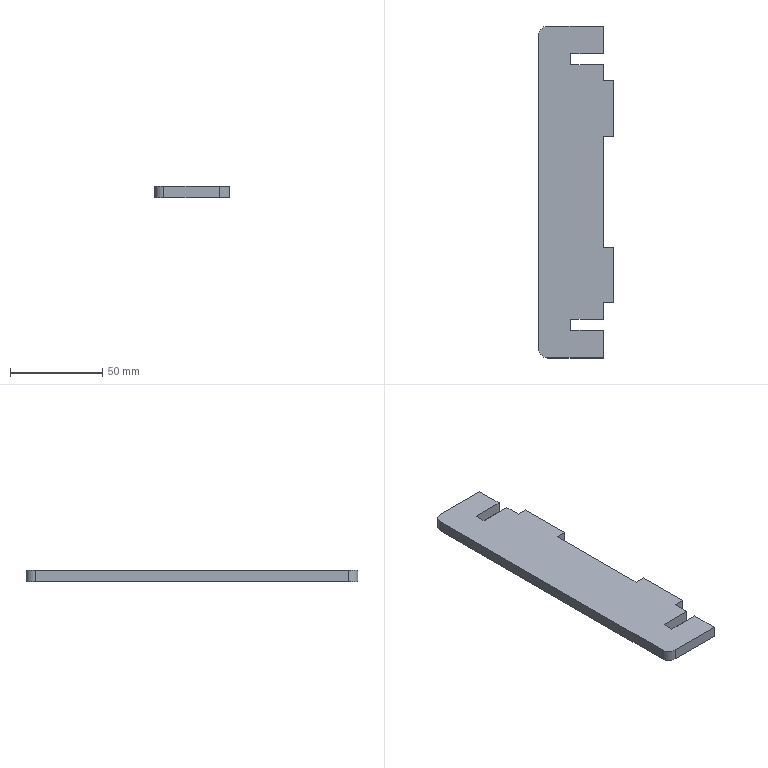Part | SolidWorks | features FlatPattern 1, SMBaseFlange 1, SheetMetal 1 | 1 solid | 24 faces | box 40.5 x 180 x 6 mm | volume 38456 mm3 | plane 22 | cylinder 2 | commonest cylinder face diameters 10 x2
STEP:
#1=CARTESIAN_POINT('',(654.3,38.691,0.));
#2=VERTEX_POINT('',#1);
#3=CARTESIAN_POINT('',(654.3,53.691,0.));
#4=VERTEX_POINT('',#3);
#5=CARTESIAN_POINT('',(654.3,53.691,0.));
#6=DIRECTION('',(0.,1.,0.));
#7=VECTOR('',#6,1000.);
#8=LINE('',#5,#7);
#9=EDGE_CURVE('',#2,#4,#8,.T.);
#10=ORIENTED_EDGE('',*,*,#9,.F.);
#11=CARTESIAN_POINT('',(654.3,38.691,-6.));
#12=VERTEX_POINT('',#11);
#13=CARTESIAN_POINT('',(654.3,38.691,-6.));
#14=DIRECTION('',(0.,0.,1.));
#15=VECTOR('',#14,1000.);
#16=LINE('',#13,#15);
#17=EDGE_CURVE('',#12,#2,#16,.T.);
#18=ORIENTED_EDGE('',*,*,#17,.F.);
#19=CARTESIAN_POINT('',(654.3,53.691,-6.));
#20=VERTEX_POINT('',#19);
#21=CARTESIAN_POINT('',(654.3,53.691,-6.));
#22=DIRECTION('',(0.,1.,0.));
#23=VECTOR('',#22,1000.);
#24=LINE('',#21,#23);
#25=EDGE_CURVE('',#12,#20,#24,.T.);
#26=ORIENTED_EDGE('',*,*,#25,.T.);
#27=CARTESIAN_POINT('',(654.3,53.691,-6.));
#28=DIRECTION('',(0.,0.,1.));
#29=VECTOR('',#28,1000.);
#30=LINE('',#27,#29);
#31=EDGE_CURVE('',#20,#4,#30,.T.);
#32=ORIENTED_EDGE('',*,*,#31,.T.);
#33=EDGE_LOOP('',(#10,#18,#26,#32));
#34=FACE_OUTER_BOUND('',#33,.T.);
#35=CARTESIAN_POINT('',(654.3,53.691,-6.));
#36=DIRECTION('',(1.,0.,0.));
#37=DIRECTION('',(0.,0.,-1.));
#38=AXIS2_PLACEMENT_3D('',#35,#36,#37);
#39=PLANE('',#38);
#40=ADVANCED_FACE('',(#34),#39,.T.);
#41=CARTESIAN_POINT('',(636.8,38.691,0.));
#42=VERTEX_POINT('',#41);
#43=CARTESIAN_POINT('',(654.3,38.691,0.));
#44=DIRECTION('',(1.,0.,0.));
#45=VECTOR('',#44,1000.);
#46=LINE('',#43,#45);
#47=EDGE_CURVE('',#42,#2,#46,.T.);
#48=ORIENTED_EDGE('',*,*,#47,.F.);
#49=CARTESIAN_POINT('',(636.8,38.691,-6.));
#50=VERTEX_POINT('',#49);
#51=CARTESIAN_POINT('',(636.8,38.691,-6.));
#52=DIRECTION('',(0.,0.,1.));
#53=VECTOR('',#52,1000.);
#54=LINE('',#51,#53);
#55=EDGE_CURVE('',#50,#42,#54,.T.);
#56=ORIENTED_EDGE('',*,*,#55,.F.);
#57=CARTESIAN_POINT('',(654.3,38.691,-6.));
#58=DIRECTION('',(1.,0.,0.));
#59=VECTOR('',#58,1000.);
#60=LINE('',#57,#59);
#61=EDGE_CURVE('',#50,#12,#60,.T.);
#62=ORIENTED_EDGE('',*,*,#61,.T.);
#63=ORIENTED_EDGE('',*,*,#17,.T.);
#64=EDGE_LOOP('',(#48,#56,#62,#63));
#65=FACE_OUTER_BOUND('',#64,.T.);
#66=CARTESIAN_POINT('',(654.3,38.691,-6.));
#67=DIRECTION('',(0.,-1.,0.));
#68=DIRECTION('',(0.,0.,-1.));
#69=AXIS2_PLACEMENT_3D('',#66,#67,#68);
#70=PLANE('',#69);
#71=ADVANCED_FACE('',(#65),#70,.T.);
#72=CARTESIAN_POINT('',(636.8,32.691,0.));
#73=VERTEX_POINT('',#72);
#74=CARTESIAN_POINT('',(636.8,38.691,0.));
#75=DIRECTION('',(0.,1.,0.));
#76=VECTOR('',#75,1000.);
#77=LINE('',#74,#76);
#78=EDGE_CURVE('',#73,#42,#77,.T.);
#79=ORIENTED_EDGE('',*,*,#78,.F.);
#80=CARTESIAN_POINT('',(636.8,32.691,-6.));
#81=VERTEX_POINT('',#80);
#82=CARTESIAN_POINT('',(636.8,32.691,-6.));
#83=DIRECTION('',(0.,0.,1.));
#84=VECTOR('',#83,1000.);
#85=LINE('',#82,#84);
#86=EDGE_CURVE('',#81,#73,#85,.T.);
#87=ORIENTED_EDGE('',*,*,#86,.F.);
#88=CARTESIAN_POINT('',(636.8,38.691,-6.));
#89=DIRECTION('',(0.,1.,0.));
#90=VECTOR('',#89,1000.);
#91=LINE('',#88,#90);
#92=EDGE_CURVE('',#81,#50,#91,.T.);
#93=ORIENTED_EDGE('',*,*,#92,.T.);
#94=ORIENTED_EDGE('',*,*,#55,.T.);
#95=EDGE_LOOP('',(#79,#87,#93,#94));
#96=FACE_OUTER_BOUND('',#95,.T.);
#97=CARTESIAN_POINT('',(636.8,38.691,-6.));
#98=DIRECTION('',(1.,0.,0.));
#99=DIRECTION('',(0.,0.,-1.));
#100=AXIS2_PLACEMENT_3D('',#97,#98,#99);
#101=PLANE('',#100);
#102=ADVANCED_FACE('',(#96),#101,.T.);
#103=CARTESIAN_POINT('',(654.3,32.691,0.));
#104=VERTEX_POINT('',#103);
#105=CARTESIAN_POINT('',(636.8,32.691,0.));
#106=DIRECTION('',(-1.,0.,0.));
#107=VECTOR('',#106,1000.);
#108=LINE('',#105,#107);
#109=EDGE_CURVE('',#104,#73,#108,.T.);
#110=ORIENTED_EDGE('',*,*,#109,.F.);
#111=CARTESIAN_POINT('',(654.3,32.691,-6.));
#112=VERTEX_POINT('',#111);
#113=CARTESIAN_POINT('',(654.3,32.691,-6.));
#114=DIRECTION('',(0.,0.,1.));
#115=VECTOR('',#114,1000.);
#116=LINE('',#113,#115);
#117=EDGE_CURVE('',#112,#104,#116,.T.);
#118=ORIENTED_EDGE('',*,*,#117,.F.);
#119=CARTESIAN_POINT('',(636.8,32.691,-6.));
#120=DIRECTION('',(-1.,0.,0.));
#121=VECTOR('',#120,1000.);
#122=LINE('',#119,#121);
#123=EDGE_CURVE('',#112,#81,#122,.T.);
#124=ORIENTED_EDGE('',*,*,#123,.T.);
#125=ORIENTED_EDGE('',*,*,#86,.T.);
#126=EDGE_LOOP('',(#110,#118,#124,#125));
#127=FACE_OUTER_BOUND('',#126,.T.);
#128=CARTESIAN_POINT('',(636.8,32.691,-6.));
#129=DIRECTION('',(0.,1.,0.));
#130=DIRECTION('',(0.,0.,1.));
#131=AXIS2_PLACEMENT_3D('',#128,#129,#130);
#132=PLANE('',#131);
#133=ADVANCED_FACE('',(#127),#132,.T.);
#134=CARTESIAN_POINT('',(654.3,23.882,0.));
#135=VERTEX_POINT('',#134);
#136=CARTESIAN_POINT('',(654.3,32.691,0.));
#137=DIRECTION('',(0.,1.,0.));
#138=VECTOR('',#137,1000.);
#139=LINE('',#136,#138);
#140=EDGE_CURVE('',#135,#104,#139,.T.);
#141=ORIENTED_EDGE('',*,*,#140,.F.);
#142=CARTESIAN_POINT('',(654.3,23.882,-6.));
#143=VERTEX_POINT('',#142);
#144=CARTESIAN_POINT('',(654.3,23.882,-6.));
#145=DIRECTION('',(0.,0.,1.));
#146=VECTOR('',#145,1000.);
#147=LINE('',#144,#146);
#148=EDGE_CURVE('',#143,#135,#147,.T.);
#149=ORIENTED_EDGE('',*,*,#148,.F.);
#150=CARTESIAN_POINT('',(654.3,32.691,-6.));
#151=DIRECTION('',(0.,1.,0.));
#152=VECTOR('',#151,1000.);
#153=LINE('',#150,#152);
#154=EDGE_CURVE('',#143,#112,#153,.T.);
#155=ORIENTED_EDGE('',*,*,#154,.T.);
#156=ORIENTED_EDGE('',*,*,#117,.T.);
#157=EDGE_LOOP('',(#141,#149,#155,#156));
#158=FACE_OUTER_BOUND('',#157,.T.);
#159=CARTESIAN_POINT('',(654.3,32.691,-6.));
#160=DIRECTION('',(1.,0.,0.));
#161=DIRECTION('',(0.,0.,-1.));
#162=AXIS2_PLACEMENT_3D('',#159,#160,#161);
#163=PLANE('',#162);
#164=ADVANCED_FACE('',(#158),#163,.T.);
#165=CARTESIAN_POINT('',(659.8,23.882,0.));
#166=VERTEX_POINT('',#165);
#167=CARTESIAN_POINT('',(659.8,23.882,0.));
#168=DIRECTION('',(-1.,0.,0.));
#169=VECTOR('',#168,1000.);
#170=LINE('',#167,#169);
#171=EDGE_CURVE('',#166,#135,#170,.T.);
#172=ORIENTED_EDGE('',*,*,#171,.F.);
#173=CARTESIAN_POINT('',(659.8,23.882,-6.));
#174=VERTEX_POINT('',#173);
#175=CARTESIAN_POINT('',(659.8,23.882,-6.));
#176=DIRECTION('',(0.,0.,1.));
#177=VECTOR('',#176,1000.);
#178=LINE('',#175,#177);
#179=EDGE_CURVE('',#174,#166,#178,.T.);
#180=ORIENTED_EDGE('',*,*,#179,.F.);
#181=CARTESIAN_POINT('',(659.8,23.882,-6.));
#182=DIRECTION('',(-1.,0.,0.));
#183=VECTOR('',#182,1000.);
#184=LINE('',#181,#183);
#185=EDGE_CURVE('',#174,#143,#184,.T.);
#186=ORIENTED_EDGE('',*,*,#185,.T.);
#187=ORIENTED_EDGE('',*,*,#148,.T.);
#188=EDGE_LOOP('',(#172,#180,#186,#187));
#189=FACE_OUTER_BOUND('',#188,.T.);
#190=CARTESIAN_POINT('',(659.8,23.882,-6.));
#191=DIRECTION('',(0.,1.,0.));
#192=DIRECTION('',(-1.,0.,0.));
#193=AXIS2_PLACEMENT_3D('',#190,#191,#192);
#194=PLANE('',#193);
#195=ADVANCED_FACE('',(#189),#194,.T.);
#196=CARTESIAN_POINT('',(659.8,-6.118,0.));
#197=VERTEX_POINT('',#196);
#198=CARTESIAN_POINT('',(659.8,-6.118,0.));
#199=DIRECTION('',(0.,1.,0.));
#200=VECTOR('',#199,1000.);
#201=LINE('',#198,#200);
#202=EDGE_CURVE('',#197,#166,#201,.T.);
#203=ORIENTED_EDGE('',*,*,#202,.F.);
#204=CARTESIAN_POINT('',(659.8,-6.118,-6.));
#205=VERTEX_POINT('',#204);
#206=CARTESIAN_POINT('',(659.8,-6.118,-6.));
#207=DIRECTION('',(0.,0.,1.));
#208=VECTOR('',#207,1000.);
#209=LINE('',#206,#208);
#210=EDGE_CURVE('',#205,#197,#209,.T.);
#211=ORIENTED_EDGE('',*,*,#210,.F.);
#212=CARTESIAN_POINT('',(659.8,-6.118,-6.));
#213=DIRECTION('',(0.,1.,0.));
#214=VECTOR('',#213,1000.);
#215=LINE('',#212,#214);
#216=EDGE_CURVE('',#205,#174,#215,.T.);
#217=ORIENTED_EDGE('',*,*,#216,.T.);
#218=ORIENTED_EDGE('',*,*,#179,.T.);
#219=EDGE_LOOP('',(#203,#211,#217,#218));
#220=FACE_OUTER_BOUND('',#219,.T.);
#221=CARTESIAN_POINT('',(659.8,-6.118,-6.));
#222=DIRECTION('',(1.,0.,0.));
#223=DIRECTION('',(0.,0.,-1.));
#224=AXIS2_PLACEMENT_3D('',#221,#222,#223);
#225=PLANE('',#224);
#226=ADVANCED_FACE('',(#220),#225,.T.);
#227=CARTESIAN_POINT('',(654.3,-6.118,0.));
#228=VERTEX_POINT('',#227);
#229=CARTESIAN_POINT('',(659.8,-6.118,0.));
#230=DIRECTION('',(1.,0.,0.));
#231=VECTOR('',#230,1000.);
#232=LINE('',#229,#231);
#233=EDGE_CURVE('',#228,#197,#232,.T.);
#234=ORIENTED_EDGE('',*,*,#233,.F.);
#235=CARTESIAN_POINT('',(654.3,-6.118,-6.));
#236=VERTEX_POINT('',#235);
#237=CARTESIAN_POINT('',(654.3,-6.118,-6.));
#238=DIRECTION('',(0.,0.,1.));
#239=VECTOR('',#238,1000.);
#240=LINE('',#237,#239);
#241=EDGE_CURVE('',#236,#228,#240,.T.);
#242=ORIENTED_EDGE('',*,*,#241,.F.);
#243=CARTESIAN_POINT('',(659.8,-6.118,-6.));
#244=DIRECTION('',(1.,0.,0.));
#245=VECTOR('',#244,1000.);
#246=LINE('',#243,#245);
#247=EDGE_CURVE('',#236,#205,#246,.T.);
#248=ORIENTED_EDGE('',*,*,#247,.T.);
#249=ORIENTED_EDGE('',*,*,#210,.T.);
#250=EDGE_LOOP('',(#234,#242,#248,#249));
#251=FACE_OUTER_BOUND('',#250,.T.);
#252=CARTESIAN_POINT('',(659.8,-6.118,-6.));
#253=DIRECTION('',(0.,-1.,0.));
#254=DIRECTION('',(1.,0.,0.));
#255=AXIS2_PLACEMENT_3D('',#252,#253,#254);
#256=PLANE('',#255);
#257=ADVANCED_FACE('',(#251),#256,.T.);
#258=CARTESIAN_POINT('',(654.3,-66.309,0.));
#259=VERTEX_POINT('',#258);
#260=CARTESIAN_POINT('',(654.3,-6.118,0.));
#261=DIRECTION('',(0.,1.,0.));
#262=VECTOR('',#261,1000.);
#263=LINE('',#260,#262);
#264=EDGE_CURVE('',#259,#228,#263,.T.);
#265=ORIENTED_EDGE('',*,*,#264,.F.);
#266=CARTESIAN_POINT('',(654.3,-66.309,-6.));
#267=VERTEX_POINT('',#266);
#268=CARTESIAN_POINT('',(654.3,-66.309,-6.));
#269=DIRECTION('',(0.,0.,1.));
#270=VECTOR('',#269,1000.);
#271=LINE('',#268,#270);
#272=EDGE_CURVE('',#267,#259,#271,.T.);
#273=ORIENTED_EDGE('',*,*,#272,.F.);
#274=CARTESIAN_POINT('',(654.3,-6.118,-6.));
#275=DIRECTION('',(0.,1.,0.));
#276=VECTOR('',#275,1000.);
#277=LINE('',#274,#276);
#278=EDGE_CURVE('',#267,#236,#277,.T.);
#279=ORIENTED_EDGE('',*,*,#278,.T.);
#280=ORIENTED_EDGE('',*,*,#241,.T.);
#281=EDGE_LOOP('',(#265,#273,#279,#280));
#282=FACE_OUTER_BOUND('',#281,.T.);
#283=CARTESIAN_POINT('',(654.3,-6.118,-6.));
#284=DIRECTION('',(1.,0.,0.));
#285=DIRECTION('',(0.,0.,-1.));
#286=AXIS2_PLACEMENT_3D('',#283,#284,#285);
#287=PLANE('',#286);
#288=ADVANCED_FACE('',(#282),#287,.T.);
#289=CARTESIAN_POINT('',(659.8,-66.309,0.));
#290=VERTEX_POINT('',#289);
#291=CARTESIAN_POINT('',(654.3,-66.309,0.));
#292=DIRECTION('',(-1.,0.,0.));
#293=VECTOR('',#292,1000.);
#294=LINE('',#291,#293);
#295=EDGE_CURVE('',#290,#259,#294,.T.);
#296=ORIENTED_EDGE('',*,*,#295,.F.);
#297=CARTESIAN_POINT('',(659.8,-66.309,-6.));
#298=VERTEX_POINT('',#297);
#299=CARTESIAN_POINT('',(659.8,-66.309,-6.));
#300=DIRECTION('',(0.,0.,1.));
#301=VECTOR('',#300,1000.);
#302=LINE('',#299,#301);
#303=EDGE_CURVE('',#298,#290,#302,.T.);
#304=ORIENTED_EDGE('',*,*,#303,.F.);
#305=CARTESIAN_POINT('',(654.3,-66.309,-6.));
#306=DIRECTION('',(-1.,0.,0.));
#307=VECTOR('',#306,1000.);
#308=LINE('',#305,#307);
#309=EDGE_CURVE('',#298,#267,#308,.T.);
#310=ORIENTED_EDGE('',*,*,#309,.T.);
#311=ORIENTED_EDGE('',*,*,#272,.T.);
#312=EDGE_LOOP('',(#296,#304,#310,#311));
#313=FACE_OUTER_BOUND('',#312,.T.);
#314=CARTESIAN_POINT('',(654.3,-66.309,-6.));
#315=DIRECTION('',(0.,1.,0.));
#316=DIRECTION('',(0.,0.,1.));
#317=AXIS2_PLACEMENT_3D('',#314,#315,#316);
#318=PLANE('',#317);
#319=ADVANCED_FACE('',(#313),#318,.T.);
#320=CARTESIAN_POINT('',(659.8,-96.309,0.));
#321=VERTEX_POINT('',#320);
#322=CARTESIAN_POINT('',(659.8,-66.309,0.));
#323=DIRECTION('',(0.,1.,0.));
#324=VECTOR('',#323,1000.);
#325=LINE('',#322,#324);
#326=EDGE_CURVE('',#321,#290,#325,.T.);
#327=ORIENTED_EDGE('',*,*,#326,.F.);
#328=CARTESIAN_POINT('',(659.8,-96.309,-6.));
#329=VERTEX_POINT('',#328);
#330=CARTESIAN_POINT('',(659.8,-96.309,-6.));
#331=DIRECTION('',(0.,0.,1.));
#332=VECTOR('',#331,1000.);
#333=LINE('',#330,#332);
#334=EDGE_CURVE('',#329,#321,#333,.T.);
#335=ORIENTED_EDGE('',*,*,#334,.F.);
#336=CARTESIAN_POINT('',(659.8,-66.309,-6.));
#337=DIRECTION('',(0.,1.,0.));
#338=VECTOR('',#337,1000.);
#339=LINE('',#336,#338);
#340=EDGE_CURVE('',#329,#298,#339,.T.);
#341=ORIENTED_EDGE('',*,*,#340,.T.);
#342=ORIENTED_EDGE('',*,*,#303,.T.);
#343=EDGE_LOOP('',(#327,#335,#341,#342));
#344=FACE_OUTER_BOUND('',#343,.T.);
#345=CARTESIAN_POINT('',(659.8,-66.309,-6.));
#346=DIRECTION('',(1.,0.,0.));
#347=DIRECTION('',(0.,0.,-1.));
#348=AXIS2_PLACEMENT_3D('',#345,#346,#347);
#349=PLANE('',#348);
#350=ADVANCED_FACE('',(#344),#349,.T.);
#351=CARTESIAN_POINT('',(654.3,-96.309,0.));
#352=VERTEX_POINT('',#351);
#353=CARTESIAN_POINT('',(659.8,-96.309,0.));
#354=DIRECTION('',(1.,0.,0.));
#355=VECTOR('',#354,1000.);
#356=LINE('',#353,#355);
#357=EDGE_CURVE('',#352,#321,#356,.T.);
#358=ORIENTED_EDGE('',*,*,#357,.F.);
#359=CARTESIAN_POINT('',(654.3,-96.309,-6.));
#360=VERTEX_POINT('',#359);
#361=CARTESIAN_POINT('',(654.3,-96.309,-6.));
#362=DIRECTION('',(0.,0.,1.));
#363=VECTOR('',#362,1000.);
#364=LINE('',#361,#363);
#365=EDGE_CURVE('',#360,#352,#364,.T.);
#366=ORIENTED_EDGE('',*,*,#365,.F.);
#367=CARTESIAN_POINT('',(659.8,-96.309,-6.));
#368=DIRECTION('',(1.,0.,0.));
#369=VECTOR('',#368,1000.);
#370=LINE('',#367,#369);
#371=EDGE_CURVE('',#360,#329,#370,.T.);
#372=ORIENTED_EDGE('',*,*,#371,.T.);
#373=ORIENTED_EDGE('',*,*,#334,.T.);
#374=EDGE_LOOP('',(#358,#366,#372,#373));
#375=FACE_OUTER_BOUND('',#374,.T.);
#376=CARTESIAN_POINT('',(659.8,-96.309,-6.));
#377=DIRECTION('',(0.,-1.,0.));
#378=DIRECTION('',(0.,0.,-1.));
#379=AXIS2_PLACEMENT_3D('',#376,#377,#378);
#380=PLANE('',#379);
#381=ADVANCED_FACE('',(#375),#380,.T.);
#382=CARTESIAN_POINT('',(654.3,-105.309,0.));
#383=VERTEX_POINT('',#382);
#384=CARTESIAN_POINT('',(654.3,-96.309,0.));
#385=DIRECTION('',(0.,1.,0.));
#386=VECTOR('',#385,1000.);
#387=LINE('',#384,#386);
#388=EDGE_CURVE('',#383,#352,#387,.T.);
#389=ORIENTED_EDGE('',*,*,#388,.F.);
#390=CARTESIAN_POINT('',(654.3,-105.309,-6.));
#391=VERTEX_POINT('',#390);
#392=CARTESIAN_POINT('',(654.3,-105.309,-6.));
#393=DIRECTION('',(0.,0.,1.));
#394=VECTOR('',#393,1000.);
#395=LINE('',#392,#394);
#396=EDGE_CURVE('',#391,#383,#395,.T.);
#397=ORIENTED_EDGE('',*,*,#396,.F.);
#398=CARTESIAN_POINT('',(654.3,-96.309,-6.));
#399=DIRECTION('',(0.,1.,0.));
#400=VECTOR('',#399,1000.);
#401=LINE('',#398,#400);
#402=EDGE_CURVE('',#391,#360,#401,.T.);
#403=ORIENTED_EDGE('',*,*,#402,.T.);
#404=ORIENTED_EDGE('',*,*,#365,.T.);
#405=EDGE_LOOP('',(#389,#397,#403,#404));
#406=FACE_OUTER_BOUND('',#405,.T.);
#407=CARTESIAN_POINT('',(654.3,-96.309,-6.));
#408=DIRECTION('',(1.,0.,0.));
#409=DIRECTION('',(0.,1.,0.));
#410=AXIS2_PLACEMENT_3D('',#407,#408,#409);
#411=PLANE('',#410);
#412=ADVANCED_FACE('',(#406),#411,.T.);
#413=CARTESIAN_POINT('',(636.8,-105.309,0.));
#414=VERTEX_POINT('',#413);
#415=CARTESIAN_POINT('',(654.3,-105.309,0.));
#416=DIRECTION('',(1.,0.,0.));
#417=VECTOR('',#416,1000.);
#418=LINE('',#415,#417);
#419=EDGE_CURVE('',#414,#383,#418,.T.);
#420=ORIENTED_EDGE('',*,*,#419,.F.);
#421=CARTESIAN_POINT('',(636.8,-105.309,-6.));
#422=VERTEX_POINT('',#421);
#423=CARTESIAN_POINT('',(636.8,-105.309,-6.));
#424=DIRECTION('',(0.,0.,1.));
#425=VECTOR('',#424,1000.);
#426=LINE('',#423,#425);
#427=EDGE_CURVE('',#422,#414,#426,.T.);
#428=ORIENTED_EDGE('',*,*,#427,.F.);
#429=CARTESIAN_POINT('',(654.3,-105.309,-6.));
#430=DIRECTION('',(1.,0.,0.));
#431=VECTOR('',#430,1000.);
#432=LINE('',#429,#431);
#433=EDGE_CURVE('',#422,#391,#432,.T.);
#434=ORIENTED_EDGE('',*,*,#433,.T.);
#435=ORIENTED_EDGE('',*,*,#396,.T.);
#436=EDGE_LOOP('',(#420,#428,#434,#435));
#437=FACE_OUTER_BOUND('',#436,.T.);
#438=CARTESIAN_POINT('',(654.3,-105.309,-6.));
#439=DIRECTION('',(0.,-1.,0.));
#440=DIRECTION('',(1.,0.,0.));
#441=AXIS2_PLACEMENT_3D('',#438,#439,#440);
#442=PLANE('',#441);
#443=ADVANCED_FACE('',(#437),#442,.T.);
#444=CARTESIAN_POINT('',(636.8,-111.309,0.));
#445=VERTEX_POINT('',#444);
#446=CARTESIAN_POINT('',(636.8,-105.309,0.));
#447=DIRECTION('',(0.,1.,0.));
#448=VECTOR('',#447,1000.);
#449=LINE('',#446,#448);
#450=EDGE_CURVE('',#445,#414,#449,.T.);
#451=ORIENTED_EDGE('',*,*,#450,.F.);
#452=CARTESIAN_POINT('',(636.8,-111.309,-6.));
#453=VERTEX_POINT('',#452);
#454=CARTESIAN_POINT('',(636.8,-111.309,-6.));
#455=DIRECTION('',(0.,0.,1.));
#456=VECTOR('',#455,1000.);
#457=LINE('',#454,#456);
#458=EDGE_CURVE('',#453,#445,#457,.T.);
#459=ORIENTED_EDGE('',*,*,#458,.F.);
#460=CARTESIAN_POINT('',(636.8,-105.309,-6.));
#461=DIRECTION('',(0.,1.,0.));
#462=VECTOR('',#461,1000.);
#463=LINE('',#460,#462);
#464=EDGE_CURVE('',#453,#422,#463,.T.);
#465=ORIENTED_EDGE('',*,*,#464,.T.);
#466=ORIENTED_EDGE('',*,*,#427,.T.);
#467=EDGE_LOOP('',(#451,#459,#465,#466));
#468=FACE_OUTER_BOUND('',#467,.T.);
#469=CARTESIAN_POINT('',(636.8,-105.309,-6.));
#470=DIRECTION('',(1.,0.,0.));
#471=DIRECTION('',(0.,0.,-1.));
#472=AXIS2_PLACEMENT_3D('',#469,#470,#471);
#473=PLANE('',#472);
#474=ADVANCED_FACE('',(#468),#473,.T.);
#475=CARTESIAN_POINT('',(654.3,-111.309,0.));
#476=VERTEX_POINT('',#475);
#477=CARTESIAN_POINT('',(636.8,-111.309,0.));
#478=DIRECTION('',(-1.,0.,0.));
#479=VECTOR('',#478,1000.);
#480=LINE('',#477,#479);
#481=EDGE_CURVE('',#476,#445,#480,.T.);
#482=ORIENTED_EDGE('',*,*,#481,.F.);
#483=CARTESIAN_POINT('',(654.3,-111.309,-6.));
#484=VERTEX_POINT('',#483);
#485=CARTESIAN_POINT('',(654.3,-111.309,-6.));
#486=DIRECTION('',(0.,0.,1.));
#487=VECTOR('',#486,1000.);
#488=LINE('',#485,#487);
#489=EDGE_CURVE('',#484,#476,#488,.T.);
#490=ORIENTED_EDGE('',*,*,#489,.F.);
#491=CARTESIAN_POINT('',(636.8,-111.309,-6.));
#492=DIRECTION('',(-1.,0.,0.));
#493=VECTOR('',#492,1000.);
#494=LINE('',#491,#493);
#495=EDGE_CURVE('',#484,#453,#494,.T.);
#496=ORIENTED_EDGE('',*,*,#495,.T.);
#497=ORIENTED_EDGE('',*,*,#458,.T.);
#498=EDGE_LOOP('',(#482,#490,#496,#497));
#499=FACE_OUTER_BOUND('',#498,.T.);
#500=CARTESIAN_POINT('',(636.8,-111.309,-6.));
#501=DIRECTION('',(0.,1.,0.));
#502=DIRECTION('',(0.,0.,1.));
#503=AXIS2_PLACEMENT_3D('',#500,#501,#502);
#504=PLANE('',#503);
#505=ADVANCED_FACE('',(#499),#504,.T.);
#506=CARTESIAN_POINT('',(654.3,-126.309,0.));
#507=VERTEX_POINT('',#506);
#508=CARTESIAN_POINT('',(654.3,-111.309,0.));
#509=DIRECTION('',(0.,1.,0.));
#510=VECTOR('',#509,1000.);
#511=LINE('',#508,#510);
#512=EDGE_CURVE('',#507,#476,#511,.T.);
#513=ORIENTED_EDGE('',*,*,#512,.F.);
#514=CARTESIAN_POINT('',(654.3,-126.309,-6.));
#515=VERTEX_POINT('',#514);
#516=CARTESIAN_POINT('',(654.3,-126.309,-6.));
#517=DIRECTION('',(0.,0.,1.));
#518=VECTOR('',#517,1000.);
#519=LINE('',#516,#518);
#520=EDGE_CURVE('',#515,#507,#519,.T.);
#521=ORIENTED_EDGE('',*,*,#520,.F.);
#522=CARTESIAN_POINT('',(654.3,-111.309,-6.));
#523=DIRECTION('',(0.,1.,0.));
#524=VECTOR('',#523,1000.);
#525=LINE('',#522,#524);
#526=EDGE_CURVE('',#515,#484,#525,.T.);
#527=ORIENTED_EDGE('',*,*,#526,.T.);
#528=ORIENTED_EDGE('',*,*,#489,.T.);
#529=EDGE_LOOP('',(#513,#521,#527,#528));
#530=FACE_OUTER_BOUND('',#529,.T.);
#531=CARTESIAN_POINT('',(654.3,-111.309,-6.));
#532=DIRECTION('',(1.,0.,0.));
#533=DIRECTION('',(0.,1.,0.));
#534=AXIS2_PLACEMENT_3D('',#531,#532,#533);
#535=PLANE('',#534);
#536=ADVANCED_FACE('',(#530),#535,.T.);
#537=CARTESIAN_POINT('',(624.3,-126.309,0.));
#538=VERTEX_POINT('',#537);
#539=CARTESIAN_POINT('',(654.3,-126.309,0.));
#540=DIRECTION('',(1.,0.,0.));
#541=VECTOR('',#540,1000.);
#542=LINE('',#539,#541);
#543=EDGE_CURVE('',#538,#507,#542,.T.);
#544=ORIENTED_EDGE('',*,*,#543,.F.);
#545=CARTESIAN_POINT('',(624.3,-126.309,-6.));
#546=VERTEX_POINT('',#545);
#547=CARTESIAN_POINT('',(624.3,-126.309,-6.));
#548=DIRECTION('',(0.,0.,1.));
#549=VECTOR('',#548,1000.);
#550=LINE('',#547,#549);
#551=EDGE_CURVE('',#546,#538,#550,.T.);
#552=ORIENTED_EDGE('',*,*,#551,.F.);
#553=CARTESIAN_POINT('',(654.3,-126.309,-6.));
#554=DIRECTION('',(1.,0.,0.));
#555=VECTOR('',#554,1000.);
#556=LINE('',#553,#555);
#557=EDGE_CURVE('',#546,#515,#556,.T.);
#558=ORIENTED_EDGE('',*,*,#557,.T.);
#559=ORIENTED_EDGE('',*,*,#520,.T.);
#560=EDGE_LOOP('',(#544,#552,#558,#559));
#561=FACE_OUTER_BOUND('',#560,.T.);
#562=CARTESIAN_POINT('',(654.3,-126.309,-6.));
#563=DIRECTION('',(0.,-1.,0.));
#564=DIRECTION('',(0.,0.,-1.));
#565=AXIS2_PLACEMENT_3D('',#562,#563,#564);
#566=PLANE('',#565);
#567=ADVANCED_FACE('',(#561),#566,.T.);
#568=CARTESIAN_POINT('',(619.3,-121.309,0.));
#569=VERTEX_POINT('',#568);
#570=CARTESIAN_POINT('',(624.3,-121.309,0.));
#571=DIRECTION('',(0.,0.,1.));
#572=DIRECTION('',(-1.,0.,0.));
#573=AXIS2_PLACEMENT_3D('',#570,#571,#572);
#574=CIRCLE('',#573,5.);
#575=EDGE_CURVE('',#569,#538,#574,.T.);
#576=ORIENTED_EDGE('',*,*,#575,.F.);
#577=CARTESIAN_POINT('',(619.3,-121.309,-6.));
#578=VERTEX_POINT('',#577);
#579=CARTESIAN_POINT('',(619.3,-121.309,-6.));
#580=DIRECTION('',(0.,0.,1.));
#581=VECTOR('',#580,1000.);
#582=LINE('',#579,#581);
#583=EDGE_CURVE('',#578,#569,#582,.T.);
#584=ORIENTED_EDGE('',*,*,#583,.F.);
#585=CARTESIAN_POINT('',(624.3,-121.309,-6.));
#586=DIRECTION('',(0.,0.,1.));
#587=DIRECTION('',(-1.,0.,0.));
#588=AXIS2_PLACEMENT_3D('',#585,#586,#587);
#589=CIRCLE('',#588,5.);
#590=EDGE_CURVE('',#578,#546,#589,.T.);
#591=ORIENTED_EDGE('',*,*,#590,.T.);
#592=ORIENTED_EDGE('',*,*,#551,.T.);
#593=EDGE_LOOP('',(#576,#584,#591,#592));
#594=FACE_OUTER_BOUND('',#593,.T.);
#595=CARTESIAN_POINT('',(624.3,-121.309,-6.));
#596=DIRECTION('',(0.,0.,1.));
#597=DIRECTION('',(1.,0.,0.));
#598=AXIS2_PLACEMENT_3D('',#595,#596,#597);
#599=CYLINDRICAL_SURFACE('',#598,5.);
#600=ADVANCED_FACE('',(#594),#599,.T.);
#601=CARTESIAN_POINT('',(619.3,48.691,0.));
#602=VERTEX_POINT('',#601);
#603=CARTESIAN_POINT('',(619.3,48.691,0.));
#604=DIRECTION('',(0.,-1.,0.));
#605=VECTOR('',#604,1000.);
#606=LINE('',#603,#605);
#607=EDGE_CURVE('',#602,#569,#606,.T.);
#608=ORIENTED_EDGE('',*,*,#607,.F.);
#609=CARTESIAN_POINT('',(619.3,48.691,-6.));
#610=VERTEX_POINT('',#609);
#611=CARTESIAN_POINT('',(619.3,48.691,-6.));
#612=DIRECTION('',(0.,0.,1.));
#613=VECTOR('',#612,1000.);
#614=LINE('',#611,#613);
#615=EDGE_CURVE('',#610,#602,#614,.T.);
#616=ORIENTED_EDGE('',*,*,#615,.F.);
#617=CARTESIAN_POINT('',(619.3,48.691,-6.));
#618=DIRECTION('',(0.,-1.,0.));
#619=VECTOR('',#618,1000.);
#620=LINE('',#617,#619);
#621=EDGE_CURVE('',#610,#578,#620,.T.);
#622=ORIENTED_EDGE('',*,*,#621,.T.);
#623=ORIENTED_EDGE('',*,*,#583,.T.);
#624=EDGE_LOOP('',(#608,#616,#622,#623));
#625=FACE_OUTER_BOUND('',#624,.T.);
#626=CARTESIAN_POINT('',(619.3,48.691,-6.));
#627=DIRECTION('',(-1.,0.,0.));
#628=DIRECTION('',(0.,0.,1.));
#629=AXIS2_PLACEMENT_3D('',#626,#627,#628);
#630=PLANE('',#629);
#631=ADVANCED_FACE('',(#625),#630,.T.);
#632=CARTESIAN_POINT('',(624.3,53.691,0.));
#633=VERTEX_POINT('',#632);
#634=CARTESIAN_POINT('',(624.3,48.691,0.));
#635=DIRECTION('',(0.,0.,1.));
#636=DIRECTION('',(1.,0.,0.));
#637=AXIS2_PLACEMENT_3D('',#634,#635,#636);
#638=CIRCLE('',#637,5.);
#639=EDGE_CURVE('',#633,#602,#638,.T.);
#640=ORIENTED_EDGE('',*,*,#639,.F.);
#641=CARTESIAN_POINT('',(624.3,53.691,-6.));
#642=VERTEX_POINT('',#641);
#643=CARTESIAN_POINT('',(624.3,53.691,-6.));
#644=DIRECTION('',(0.,0.,1.));
#645=VECTOR('',#644,1000.);
#646=LINE('',#643,#645);
#647=EDGE_CURVE('',#642,#633,#646,.T.);
#648=ORIENTED_EDGE('',*,*,#647,.F.);
#649=CARTESIAN_POINT('',(624.3,48.691,-6.));
#650=DIRECTION('',(0.,0.,1.));
#651=DIRECTION('',(1.,0.,0.));
#652=AXIS2_PLACEMENT_3D('',#649,#650,#651);
#653=CIRCLE('',#652,5.);
#654=EDGE_CURVE('',#642,#610,#653,.T.);
#655=ORIENTED_EDGE('',*,*,#654,.T.);
#656=ORIENTED_EDGE('',*,*,#615,.T.);
#657=EDGE_LOOP('',(#640,#648,#655,#656));
#658=FACE_OUTER_BOUND('',#657,.T.);
#659=CARTESIAN_POINT('',(624.3,48.691,-6.));
#660=DIRECTION('',(0.,0.,1.));
#661=DIRECTION('',(1.,0.,0.));
#662=AXIS2_PLACEMENT_3D('',#659,#660,#661);
#663=CYLINDRICAL_SURFACE('',#662,5.);
#664=ADVANCED_FACE('',(#658),#663,.T.);
#665=CARTESIAN_POINT('',(654.3,53.691,0.));
#666=DIRECTION('',(-1.,0.,0.));
#667=VECTOR('',#666,1000.);
#668=LINE('',#665,#667);
#669=EDGE_CURVE('',#4,#633,#668,.T.);
#670=ORIENTED_EDGE('',*,*,#669,.F.);
#671=ORIENTED_EDGE('',*,*,#31,.F.);
#672=CARTESIAN_POINT('',(654.3,53.691,-6.));
#673=DIRECTION('',(-1.,0.,0.));
#674=VECTOR('',#673,1000.);
#675=LINE('',#672,#674);
#676=EDGE_CURVE('',#20,#642,#675,.T.);
#677=ORIENTED_EDGE('',*,*,#676,.T.);
#678=ORIENTED_EDGE('',*,*,#647,.T.);
#679=EDGE_LOOP('',(#670,#671,#677,#678));
#680=FACE_OUTER_BOUND('',#679,.T.);
#681=CARTESIAN_POINT('',(654.3,53.691,-6.));
#682=DIRECTION('',(0.,1.,0.));
#683=DIRECTION('',(-1.,0.,0.));
#684=AXIS2_PLACEMENT_3D('',#681,#682,#683);
#685=PLANE('',#684);
#686=ADVANCED_FACE('',(#680),#685,.T.);
#687=ORIENTED_EDGE('',*,*,#25,.F.);
#688=ORIENTED_EDGE('',*,*,#61,.F.);
#689=ORIENTED_EDGE('',*,*,#92,.F.);
#690=ORIENTED_EDGE('',*,*,#123,.F.);
#691=ORIENTED_EDGE('',*,*,#154,.F.);
#692=ORIENTED_EDGE('',*,*,#185,.F.);
#693=ORIENTED_EDGE('',*,*,#216,.F.);
#694=ORIENTED_EDGE('',*,*,#247,.F.);
#695=ORIENTED_EDGE('',*,*,#278,.F.);
#696=ORIENTED_EDGE('',*,*,#309,.F.);
#697=ORIENTED_EDGE('',*,*,#340,.F.);
#698=ORIENTED_EDGE('',*,*,#371,.F.);
#699=ORIENTED_EDGE('',*,*,#402,.F.);
#700=ORIENTED_EDGE('',*,*,#433,.F.);
#701=ORIENTED_EDGE('',*,*,#464,.F.);
#702=ORIENTED_EDGE('',*,*,#495,.F.);
#703=ORIENTED_EDGE('',*,*,#526,.F.);
#704=ORIENTED_EDGE('',*,*,#557,.F.);
#705=ORIENTED_EDGE('',*,*,#590,.F.);
#706=ORIENTED_EDGE('',*,*,#621,.F.);
#707=ORIENTED_EDGE('',*,*,#654,.F.);
#708=ORIENTED_EDGE('',*,*,#676,.F.);
#709=EDGE_LOOP('',(#687,#688,#689,#690,#691,#692,#693,#694,#695,#696,#697,#698,#699,#700,#701,#702,#703,#704,#705,#706,#707,#708));
#710=FACE_OUTER_BOUND('',#709,.T.);
#711=CARTESIAN_POINT('',(624.3,-121.309,-6.));
#712=DIRECTION('',(0.,0.,-1.));
#713=DIRECTION('',(-1.,0.,0.));
#714=AXIS2_PLACEMENT_3D('',#711,#712,#713);
#715=PLANE('',#714);
#716=ADVANCED_FACE('',(#710),#715,.T.);
#717=ORIENTED_EDGE('',*,*,#9,.T.);
#718=ORIENTED_EDGE('',*,*,#669,.T.);
#719=ORIENTED_EDGE('',*,*,#639,.T.);
#720=ORIENTED_EDGE('',*,*,#607,.T.);
#721=ORIENTED_EDGE('',*,*,#575,.T.);
#722=ORIENTED_EDGE('',*,*,#543,.T.);
#723=ORIENTED_EDGE('',*,*,#512,.T.);
#724=ORIENTED_EDGE('',*,*,#481,.T.);
#725=ORIENTED_EDGE('',*,*,#450,.T.);
#726=ORIENTED_EDGE('',*,*,#419,.T.);
#727=ORIENTED_EDGE('',*,*,#388,.T.);
#728=ORIENTED_EDGE('',*,*,#357,.T.);
#729=ORIENTED_EDGE('',*,*,#326,.T.);
#730=ORIENTED_EDGE('',*,*,#295,.T.);
#731=ORIENTED_EDGE('',*,*,#264,.T.);
#732=ORIENTED_EDGE('',*,*,#233,.T.);
#733=ORIENTED_EDGE('',*,*,#202,.T.);
#734=ORIENTED_EDGE('',*,*,#171,.T.);
#735=ORIENTED_EDGE('',*,*,#140,.T.);
#736=ORIENTED_EDGE('',*,*,#109,.T.);
#737=ORIENTED_EDGE('',*,*,#78,.T.);
#738=ORIENTED_EDGE('',*,*,#47,.T.);
#739=EDGE_LOOP('',(#717,#718,#719,#720,#721,#722,#723,#724,#725,#726,#727,#728,#729,#730,#731,#732,#733,#734,#735,#736,#737,#738));
#740=FACE_OUTER_BOUND('',#739,.T.);
#741=CARTESIAN_POINT('',(624.3,-121.309,0.));
#742=DIRECTION('',(0.,0.,-1.));
#743=DIRECTION('',(-1.,0.,0.));
#744=AXIS2_PLACEMENT_3D('',#741,#742,#743);
#745=PLANE('',#744);
#746=ADVANCED_FACE('',(#740),#745,.F.);
#747=CLOSED_SHELL('',(#40,#71,#102,#133,#164,#195,#226,#257,#288,#319,#350,#381,#412,#443,#474,#505,#536,#567,#600,#631,#664,#686,#716,#746));
#748=MANIFOLD_SOLID_BREP('',#747);
#749=CARTESIAN_POINT('',(0.,0.,0.));
#750=DIRECTION('',(0.,0.,1.));
#751=DIRECTION('',(1.,0.,0.));
#752=AXIS2_PLACEMENT_3D('',#749,#750,#751);
#753=(LENGTH_UNIT()NAMED_UNIT(*)SI_UNIT(.MILLI.,.METRE.));
#754=UNCERTAINTY_MEASURE_WITH_UNIT(LENGTH_MEASURE(0.00001),#753,'','');
#755=(NAMED_UNIT(*)PLANE_ANGLE_UNIT()SI_UNIT($,.RADIAN.));
#756=(NAMED_UNIT(*)SI_UNIT($,.STERADIAN.)SOLID_ANGLE_UNIT());
#757=(GEOMETRIC_REPRESENTATION_CONTEXT(3)GLOBAL_UNCERTAINTY_ASSIGNED_CONTEXT((#754))GLOBAL_UNIT_ASSIGNED_CONTEXT((#753,#755,#756))REPRESENTATION_CONTEXT('',''));
#758=ADVANCED_BREP_SHAPE_REPRESENTATION('',(#748,#752),#757);